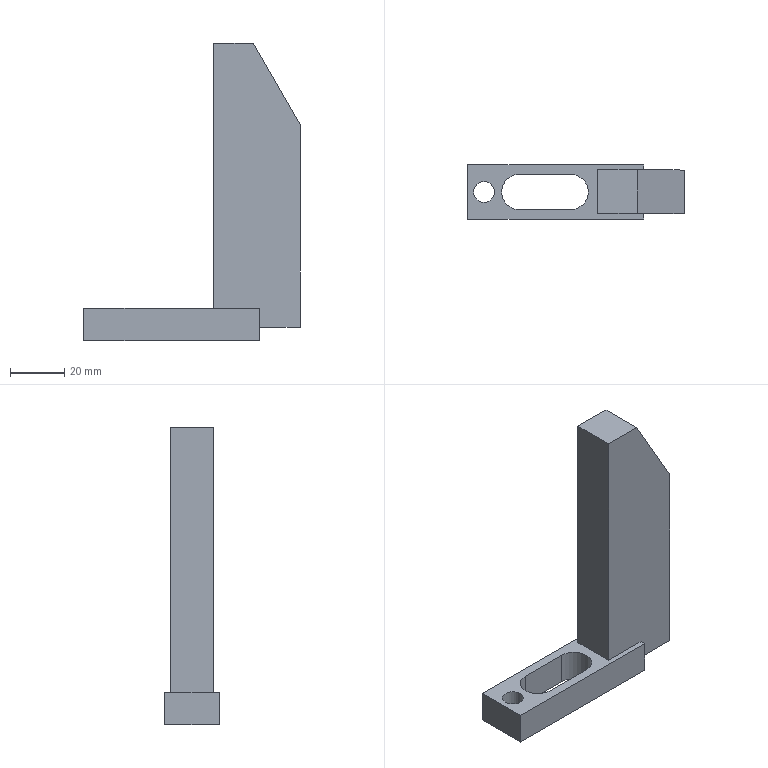Part | NX | features solid 2 | 1 solid | 18 faces | box 80 x 20 x 110 mm | volume 58169 mm3 | plane 15 | cylinder 3 | commonest cylinder face diameters 13 x2 7.8 x1
STEP:
#1=CARTESIAN_POINT('',(-633.,83.,-110.));
#2=VERTEX_POINT('',#1);
#3=CARTESIAN_POINT('',(-633.,83.,-103.));
#4=VERTEX_POINT('',#3);
#5=CARTESIAN_POINT('',(-633.,83.,-85.));
#6=DIRECTION('',(0.,0.,1.));
#7=VECTOR('',#6,1000.);
#8=LINE('',#5,#7);
#9=EDGE_CURVE('',#2,#4,#8,.T.);
#10=ORIENTED_EDGE('',*,*,#9,.T.);
#11=CARTESIAN_POINT('',(-650.,83.,-103.));
#12=VERTEX_POINT('',#11);
#13=CARTESIAN_POINT('',(-665.5,83.,-103.));
#14=DIRECTION('',(-1.,0.,0.));
#15=VECTOR('',#14,1000.);
#16=LINE('',#13,#15);
#17=EDGE_CURVE('',#4,#12,#16,.T.);
#18=ORIENTED_EDGE('',*,*,#17,.T.);
#19=CARTESIAN_POINT('',(-650.,83.,-5.));
#20=VERTEX_POINT('',#19);
#21=CARTESIAN_POINT('',(-650.,83.,-150.));
#22=DIRECTION('',(0.,0.,1.));
#23=VECTOR('',#22,1000.);
#24=LINE('',#21,#23);
#25=EDGE_CURVE('',#12,#20,#24,.T.);
#26=ORIENTED_EDGE('',*,*,#25,.T.);
#27=CARTESIAN_POINT('',(-635.321,83.,-5.));
#28=VERTEX_POINT('',#27);
#29=CARTESIAN_POINT('',(-634.,83.,-5.));
#30=DIRECTION('',(1.,0.,0.));
#31=VECTOR('',#30,1000.);
#32=LINE('',#29,#31);
#33=EDGE_CURVE('',#20,#28,#32,.T.);
#34=ORIENTED_EDGE('',*,*,#33,.T.);
#35=CARTESIAN_POINT('',(-618.,83.,-35.));
#36=VERTEX_POINT('',#35);
#37=CARTESIAN_POINT('',(-618.,83.,-35.));
#38=DIRECTION('',(-0.5,0.,0.866));
#39=VECTOR('',#38,1000.);
#40=LINE('',#37,#39);
#41=EDGE_CURVE('',#36,#28,#40,.T.);
#42=ORIENTED_EDGE('',*,*,#41,.F.);
#43=CARTESIAN_POINT('',(-618.,83.,-110.));
#44=VERTEX_POINT('',#43);
#45=CARTESIAN_POINT('',(-618.,83.,-80.));
#46=DIRECTION('',(0.,0.,1.));
#47=VECTOR('',#46,1000.);
#48=LINE('',#45,#47);
#49=EDGE_CURVE('',#44,#36,#48,.T.);
#50=ORIENTED_EDGE('',*,*,#49,.F.);
#51=CARTESIAN_POINT('',(-634.,83.,-110.));
#52=DIRECTION('',(-1.,0.,0.));
#53=VECTOR('',#52,1000.);
#54=LINE('',#51,#53);
#55=EDGE_CURVE('',#44,#2,#54,.T.);
#56=ORIENTED_EDGE('',*,*,#55,.T.);
#57=EDGE_LOOP('',(#10,#18,#26,#34,#42,#50,#56));
#58=FACE_BOUND('',#57,.T.);
#59=CARTESIAN_POINT('',(-634.,83.,-80.));
#60=DIRECTION('',(0.,1.,0.));
#61=DIRECTION('',(0.,0.,-1.));
#62=AXIS2_PLACEMENT_3D('',#59,#60,#61);
#63=PLANE('',#62);
#64=ADVANCED_FACE('',(#58),#63,.T.);
#65=ORIENTED_EDGE('',*,*,#49,.T.);
#66=CARTESIAN_POINT('',(-618.,67.,-35.));
#67=VERTEX_POINT('',#66);
#68=CARTESIAN_POINT('',(-618.,75.,-35.));
#69=DIRECTION('',(0.,-1.,0.));
#70=VECTOR('',#69,1000.);
#71=LINE('',#68,#70);
#72=EDGE_CURVE('',#36,#67,#71,.T.);
#73=ORIENTED_EDGE('',*,*,#72,.T.);
#74=CARTESIAN_POINT('',(-618.,67.,-110.));
#75=VERTEX_POINT('',#74);
#76=CARTESIAN_POINT('',(-618.,67.,-80.));
#77=DIRECTION('',(0.,0.,1.));
#78=VECTOR('',#77,1000.);
#79=LINE('',#76,#78);
#80=EDGE_CURVE('',#75,#67,#79,.T.);
#81=ORIENTED_EDGE('',*,*,#80,.F.);
#82=CARTESIAN_POINT('',(-618.,75.,-110.));
#83=DIRECTION('',(0.,1.,0.));
#84=VECTOR('',#83,1000.);
#85=LINE('',#82,#84);
#86=EDGE_CURVE('',#75,#44,#85,.T.);
#87=ORIENTED_EDGE('',*,*,#86,.T.);
#88=EDGE_LOOP('',(#65,#73,#81,#87));
#89=FACE_BOUND('',#88,.T.);
#90=CARTESIAN_POINT('',(-618.,75.,-80.));
#91=DIRECTION('',(1.,0.,0.));
#92=DIRECTION('',(0.,0.,1.));
#93=AXIS2_PLACEMENT_3D('',#90,#91,#92);
#94=PLANE('',#93);
#95=ADVANCED_FACE('',(#89),#94,.T.);
#96=ORIENTED_EDGE('',*,*,#80,.T.);
#97=CARTESIAN_POINT('',(-635.321,67.,-5.));
#98=VERTEX_POINT('',#97);
#99=CARTESIAN_POINT('',(-618.,67.,-35.));
#100=DIRECTION('',(-0.5,0.,0.866));
#101=VECTOR('',#100,1000.);
#102=LINE('',#99,#101);
#103=EDGE_CURVE('',#67,#98,#102,.T.);
#104=ORIENTED_EDGE('',*,*,#103,.T.);
#105=CARTESIAN_POINT('',(-650.,67.,-5.));
#106=VERTEX_POINT('',#105);
#107=CARTESIAN_POINT('',(-634.,67.,-5.));
#108=DIRECTION('',(-1.,0.,0.));
#109=VECTOR('',#108,1000.);
#110=LINE('',#107,#109);
#111=EDGE_CURVE('',#98,#106,#110,.T.);
#112=ORIENTED_EDGE('',*,*,#111,.T.);
#113=CARTESIAN_POINT('',(-650.,67.,-103.));
#114=VERTEX_POINT('',#113);
#115=CARTESIAN_POINT('',(-650.,67.,-150.));
#116=DIRECTION('',(0.,0.,1.));
#117=VECTOR('',#116,1000.);
#118=LINE('',#115,#117);
#119=EDGE_CURVE('',#114,#106,#118,.T.);
#120=ORIENTED_EDGE('',*,*,#119,.F.);
#121=CARTESIAN_POINT('',(-633.,67.,-103.));
#122=VERTEX_POINT('',#121);
#123=CARTESIAN_POINT('',(-665.5,67.,-103.));
#124=DIRECTION('',(1.,0.,0.));
#125=VECTOR('',#124,1000.);
#126=LINE('',#123,#125);
#127=EDGE_CURVE('',#114,#122,#126,.T.);
#128=ORIENTED_EDGE('',*,*,#127,.T.);
#129=CARTESIAN_POINT('',(-633.,67.,-110.));
#130=VERTEX_POINT('',#129);
#131=CARTESIAN_POINT('',(-633.,67.,-85.));
#132=DIRECTION('',(0.,0.,-1.));
#133=VECTOR('',#132,1000.);
#134=LINE('',#131,#133);
#135=EDGE_CURVE('',#122,#130,#134,.T.);
#136=ORIENTED_EDGE('',*,*,#135,.T.);
#137=CARTESIAN_POINT('',(-634.,67.,-110.));
#138=DIRECTION('',(1.,0.,0.));
#139=VECTOR('',#138,1000.);
#140=LINE('',#137,#139);
#141=EDGE_CURVE('',#130,#75,#140,.T.);
#142=ORIENTED_EDGE('',*,*,#141,.T.);
#143=EDGE_LOOP('',(#96,#104,#112,#120,#128,#136,#142));
#144=FACE_BOUND('',#143,.T.);
#145=CARTESIAN_POINT('',(-634.,67.,-80.));
#146=DIRECTION('',(0.,-1.,0.));
#147=DIRECTION('',(0.,0.,1.));
#148=AXIS2_PLACEMENT_3D('',#145,#146,#147);
#149=PLANE('',#148);
#150=ADVANCED_FACE('',(#144),#149,.T.);
#151=ORIENTED_EDGE('',*,*,#127,.F.);
#152=CARTESIAN_POINT('',(-650.,75.,-103.));
#153=DIRECTION('',(0.,-1.,0.));
#154=VECTOR('',#153,1000.);
#155=LINE('',#152,#154);
#156=EDGE_CURVE('',#12,#114,#155,.T.);
#157=ORIENTED_EDGE('',*,*,#156,.F.);
#158=ORIENTED_EDGE('',*,*,#17,.F.);
#159=CARTESIAN_POINT('',(-633.,85.,-103.));
#160=VERTEX_POINT('',#159);
#161=CARTESIAN_POINT('',(-633.,75.,-103.));
#162=DIRECTION('',(0.,-1.,0.));
#163=VECTOR('',#162,1000.);
#164=LINE('',#161,#163);
#165=EDGE_CURVE('',#160,#4,#164,.T.);
#166=ORIENTED_EDGE('',*,*,#165,.F.);
#167=CARTESIAN_POINT('',(-698.,85.,-103.));
#168=VERTEX_POINT('',#167);
#169=CARTESIAN_POINT('',(-665.5,85.,-103.));
#170=DIRECTION('',(1.,0.,0.));
#171=VECTOR('',#170,1000.);
#172=LINE('',#169,#171);
#173=EDGE_CURVE('',#168,#160,#172,.T.);
#174=ORIENTED_EDGE('',*,*,#173,.F.);
#175=CARTESIAN_POINT('',(-698.,65.,-103.));
#176=VERTEX_POINT('',#175);
#177=CARTESIAN_POINT('',(-698.,75.,-103.));
#178=DIRECTION('',(0.,1.,0.));
#179=VECTOR('',#178,1000.);
#180=LINE('',#177,#179);
#181=EDGE_CURVE('',#176,#168,#180,.T.);
#182=ORIENTED_EDGE('',*,*,#181,.F.);
#183=CARTESIAN_POINT('',(-633.,65.,-103.));
#184=VERTEX_POINT('',#183);
#185=CARTESIAN_POINT('',(-665.5,65.,-103.));
#186=DIRECTION('',(-1.,0.,0.));
#187=VECTOR('',#186,1000.);
#188=LINE('',#185,#187);
#189=EDGE_CURVE('',#184,#176,#188,.T.);
#190=ORIENTED_EDGE('',*,*,#189,.F.);
#191=CARTESIAN_POINT('',(-633.,75.,-103.));
#192=DIRECTION('',(0.,-1.,0.));
#193=VECTOR('',#192,1000.);
#194=LINE('',#191,#193);
#195=EDGE_CURVE('',#122,#184,#194,.T.);
#196=ORIENTED_EDGE('',*,*,#195,.F.);
#197=EDGE_LOOP('',(#151,#157,#158,#166,#174,#182,#190,#196));
#198=FACE_BOUND('',#197,.T.);
#199=CARTESIAN_POINT('',(-660.,81.5,-103.));
#200=VERTEX_POINT('',#199);
#201=CARTESIAN_POINT('',(-660.,68.5,-103.));
#202=VERTEX_POINT('',#201);
#203=CARTESIAN_POINT('',(-660.,75.,-103.));
#204=DIRECTION('',(0.,0.,-1.));
#205=DIRECTION('',(1.,0.,0.));
#206=AXIS2_PLACEMENT_3D('',#203,#204,#205);
#207=CIRCLE('',#206,6.5);
#208=EDGE_CURVE('',#200,#202,#207,.T.);
#209=ORIENTED_EDGE('',*,*,#208,.T.);
#210=CARTESIAN_POINT('',(-679.,68.5,-103.));
#211=VERTEX_POINT('',#210);
#212=CARTESIAN_POINT('',(-669.5,68.5,-103.));
#213=DIRECTION('',(-1.,0.,0.));
#214=VECTOR('',#213,1000.);
#215=LINE('',#212,#214);
#216=EDGE_CURVE('',#202,#211,#215,.T.);
#217=ORIENTED_EDGE('',*,*,#216,.T.);
#218=CARTESIAN_POINT('',(-679.,81.5,-103.));
#219=VERTEX_POINT('',#218);
#220=CARTESIAN_POINT('',(-679.,75.,-103.));
#221=DIRECTION('',(0.,0.,-1.));
#222=DIRECTION('',(1.,0.,0.));
#223=AXIS2_PLACEMENT_3D('',#220,#221,#222);
#224=CIRCLE('',#223,6.5);
#225=EDGE_CURVE('',#211,#219,#224,.T.);
#226=ORIENTED_EDGE('',*,*,#225,.T.);
#227=CARTESIAN_POINT('',(-669.5,81.5,-103.));
#228=DIRECTION('',(1.,0.,0.));
#229=VECTOR('',#228,1000.);
#230=LINE('',#227,#229);
#231=EDGE_CURVE('',#219,#200,#230,.T.);
#232=ORIENTED_EDGE('',*,*,#231,.T.);
#233=EDGE_LOOP('',(#209,#217,#226,#232));
#234=FACE_BOUND('',#233,.T.);
#235=CARTESIAN_POINT('',(-688.1,75.,-103.));
#236=VERTEX_POINT('',#235);
#237=CARTESIAN_POINT('',(-692.,75.,-103.));
#238=DIRECTION('',(0.,0.,-1.));
#239=DIRECTION('',(1.,0.,0.));
#240=AXIS2_PLACEMENT_3D('',#237,#238,#239);
#241=CIRCLE('',#240,3.9);
#242=EDGE_CURVE('',#236,#236,#241,.T.);
#243=ORIENTED_EDGE('',*,*,#242,.T.);
#244=EDGE_LOOP('',(#243));
#245=FACE_BOUND('',#244,.T.);
#246=CARTESIAN_POINT('',(-665.5,75.,-103.));
#247=DIRECTION('',(0.,0.,1.));
#248=DIRECTION('',(-1.,0.,0.));
#249=AXIS2_PLACEMENT_3D('',#246,#247,#248);
#250=PLANE('',#249);
#251=ADVANCED_FACE('',(#198,#234,#245),#250,.T.);
#252=CARTESIAN_POINT('',(-698.,85.,-115.));
#253=VERTEX_POINT('',#252);
#254=CARTESIAN_POINT('',(-698.,85.,-85.));
#255=DIRECTION('',(0.,0.,1.));
#256=VECTOR('',#255,1000.);
#257=LINE('',#254,#256);
#258=EDGE_CURVE('',#253,#168,#257,.T.);
#259=ORIENTED_EDGE('',*,*,#258,.T.);
#260=ORIENTED_EDGE('',*,*,#173,.T.);
#261=CARTESIAN_POINT('',(-633.,85.,-115.));
#262=VERTEX_POINT('',#261);
#263=CARTESIAN_POINT('',(-633.,85.,-85.));
#264=DIRECTION('',(0.,0.,1.));
#265=VECTOR('',#264,1000.);
#266=LINE('',#263,#265);
#267=EDGE_CURVE('',#262,#160,#266,.T.);
#268=ORIENTED_EDGE('',*,*,#267,.F.);
#269=CARTESIAN_POINT('',(-665.5,85.,-115.));
#270=DIRECTION('',(-1.,0.,0.));
#271=VECTOR('',#270,1000.);
#272=LINE('',#269,#271);
#273=EDGE_CURVE('',#262,#253,#272,.T.);
#274=ORIENTED_EDGE('',*,*,#273,.T.);
#275=EDGE_LOOP('',(#259,#260,#268,#274));
#276=FACE_BOUND('',#275,.T.);
#277=CARTESIAN_POINT('',(-665.5,85.,-85.));
#278=DIRECTION('',(0.,1.,0.));
#279=DIRECTION('',(0.,0.,-1.));
#280=AXIS2_PLACEMENT_3D('',#277,#278,#279);
#281=PLANE('',#280);
#282=ADVANCED_FACE('',(#276),#281,.T.);
#283=ORIENTED_EDGE('',*,*,#9,.F.);
#284=CARTESIAN_POINT('',(-633.,75.,-110.));
#285=DIRECTION('',(0.,1.,0.));
#286=VECTOR('',#285,1000.);
#287=LINE('',#284,#286);
#288=EDGE_CURVE('',#130,#2,#287,.T.);
#289=ORIENTED_EDGE('',*,*,#288,.F.);
#290=ORIENTED_EDGE('',*,*,#135,.F.);
#291=ORIENTED_EDGE('',*,*,#195,.T.);
#292=CARTESIAN_POINT('',(-633.,65.,-115.));
#293=VERTEX_POINT('',#292);
#294=CARTESIAN_POINT('',(-633.,65.,-85.));
#295=DIRECTION('',(0.,0.,1.));
#296=VECTOR('',#295,1000.);
#297=LINE('',#294,#296);
#298=EDGE_CURVE('',#293,#184,#297,.T.);
#299=ORIENTED_EDGE('',*,*,#298,.F.);
#300=CARTESIAN_POINT('',(-633.,75.,-115.));
#301=DIRECTION('',(0.,1.,0.));
#302=VECTOR('',#301,1000.);
#303=LINE('',#300,#302);
#304=EDGE_CURVE('',#293,#262,#303,.T.);
#305=ORIENTED_EDGE('',*,*,#304,.T.);
#306=ORIENTED_EDGE('',*,*,#267,.T.);
#307=ORIENTED_EDGE('',*,*,#165,.T.);
#308=EDGE_LOOP('',(#283,#289,#290,#291,#299,#305,#306,#307));
#309=FACE_BOUND('',#308,.T.);
#310=CARTESIAN_POINT('',(-633.,75.,-85.));
#311=DIRECTION('',(1.,0.,0.));
#312=DIRECTION('',(0.,0.,1.));
#313=AXIS2_PLACEMENT_3D('',#310,#311,#312);
#314=PLANE('',#313);
#315=ADVANCED_FACE('',(#309),#314,.T.);
#316=ORIENTED_EDGE('',*,*,#298,.T.);
#317=ORIENTED_EDGE('',*,*,#189,.T.);
#318=CARTESIAN_POINT('',(-698.,65.,-115.));
#319=VERTEX_POINT('',#318);
#320=CARTESIAN_POINT('',(-698.,65.,-85.));
#321=DIRECTION('',(0.,0.,1.));
#322=VECTOR('',#321,1000.);
#323=LINE('',#320,#322);
#324=EDGE_CURVE('',#319,#176,#323,.T.);
#325=ORIENTED_EDGE('',*,*,#324,.F.);
#326=CARTESIAN_POINT('',(-665.5,65.,-115.));
#327=DIRECTION('',(1.,0.,0.));
#328=VECTOR('',#327,1000.);
#329=LINE('',#326,#328);
#330=EDGE_CURVE('',#319,#293,#329,.T.);
#331=ORIENTED_EDGE('',*,*,#330,.T.);
#332=EDGE_LOOP('',(#316,#317,#325,#331));
#333=FACE_BOUND('',#332,.T.);
#334=CARTESIAN_POINT('',(-665.5,65.,-85.));
#335=DIRECTION('',(0.,-1.,0.));
#336=DIRECTION('',(0.,0.,1.));
#337=AXIS2_PLACEMENT_3D('',#334,#335,#336);
#338=PLANE('',#337);
#339=ADVANCED_FACE('',(#333),#338,.T.);
#340=CARTESIAN_POINT('',(-660.,68.5,-115.));
#341=VERTEX_POINT('',#340);
#342=CARTESIAN_POINT('',(-660.,81.5,-115.));
#343=VERTEX_POINT('',#342);
#344=CARTESIAN_POINT('',(-660.,75.,-115.));
#345=DIRECTION('',(0.,0.,1.));
#346=DIRECTION('',(-1.,0.,0.));
#347=AXIS2_PLACEMENT_3D('',#344,#345,#346);
#348=CIRCLE('',#347,6.5);
#349=EDGE_CURVE('',#341,#343,#348,.T.);
#350=ORIENTED_EDGE('',*,*,#349,.T.);
#351=CARTESIAN_POINT('',(-679.,81.5,-115.));
#352=VERTEX_POINT('',#351);
#353=CARTESIAN_POINT('',(-669.5,81.5,-115.));
#354=DIRECTION('',(-1.,0.,0.));
#355=VECTOR('',#354,1000.);
#356=LINE('',#353,#355);
#357=EDGE_CURVE('',#343,#352,#356,.T.);
#358=ORIENTED_EDGE('',*,*,#357,.T.);
#359=CARTESIAN_POINT('',(-679.,68.5,-115.));
#360=VERTEX_POINT('',#359);
#361=CARTESIAN_POINT('',(-679.,75.,-115.));
#362=DIRECTION('',(0.,0.,1.));
#363=DIRECTION('',(-1.,0.,0.));
#364=AXIS2_PLACEMENT_3D('',#361,#362,#363);
#365=CIRCLE('',#364,6.5);
#366=EDGE_CURVE('',#352,#360,#365,.T.);
#367=ORIENTED_EDGE('',*,*,#366,.T.);
#368=CARTESIAN_POINT('',(-669.5,68.5,-115.));
#369=DIRECTION('',(1.,0.,0.));
#370=VECTOR('',#369,1000.);
#371=LINE('',#368,#370);
#372=EDGE_CURVE('',#360,#341,#371,.T.);
#373=ORIENTED_EDGE('',*,*,#372,.T.);
#374=EDGE_LOOP('',(#350,#358,#367,#373));
#375=FACE_BOUND('',#374,.T.);
#376=CARTESIAN_POINT('',(-695.9,75.,-115.));
#377=VERTEX_POINT('',#376);
#378=CARTESIAN_POINT('',(-692.,75.,-115.));
#379=DIRECTION('',(0.,0.,1.));
#380=DIRECTION('',(-1.,0.,0.));
#381=AXIS2_PLACEMENT_3D('',#378,#379,#380);
#382=CIRCLE('',#381,3.9);
#383=EDGE_CURVE('',#377,#377,#382,.T.);
#384=ORIENTED_EDGE('',*,*,#383,.T.);
#385=EDGE_LOOP('',(#384));
#386=FACE_BOUND('',#385,.T.);
#387=CARTESIAN_POINT('',(-698.,75.,-115.));
#388=DIRECTION('',(0.,-1.,0.));
#389=VECTOR('',#388,1000.);
#390=LINE('',#387,#389);
#391=EDGE_CURVE('',#253,#319,#390,.T.);
#392=ORIENTED_EDGE('',*,*,#391,.F.);
#393=ORIENTED_EDGE('',*,*,#273,.F.);
#394=ORIENTED_EDGE('',*,*,#304,.F.);
#395=ORIENTED_EDGE('',*,*,#330,.F.);
#396=EDGE_LOOP('',(#392,#393,#394,#395));
#397=FACE_BOUND('',#396,.T.);
#398=CARTESIAN_POINT('',(-665.5,75.,-115.));
#399=DIRECTION('',(0.,0.,-1.));
#400=DIRECTION('',(1.,0.,0.));
#401=AXIS2_PLACEMENT_3D('',#398,#399,#400);
#402=PLANE('',#401);
#403=ADVANCED_FACE('',(#375,#386,#397),#402,.T.);
#404=ORIENTED_EDGE('',*,*,#391,.T.);
#405=ORIENTED_EDGE('',*,*,#324,.T.);
#406=ORIENTED_EDGE('',*,*,#181,.T.);
#407=ORIENTED_EDGE('',*,*,#258,.F.);
#408=EDGE_LOOP('',(#404,#405,#406,#407));
#409=FACE_BOUND('',#408,.T.);
#410=CARTESIAN_POINT('',(-698.,75.,-85.));
#411=DIRECTION('',(-1.,0.,0.));
#412=DIRECTION('',(0.,0.,-1.));
#413=AXIS2_PLACEMENT_3D('',#410,#411,#412);
#414=PLANE('',#413);
#415=ADVANCED_FACE('',(#409),#414,.T.);
#416=ORIENTED_EDGE('',*,*,#242,.F.);
#417=EDGE_LOOP('',(#416));
#418=FACE_BOUND('',#417,.T.);
#419=ORIENTED_EDGE('',*,*,#383,.F.);
#420=EDGE_LOOP('',(#419));
#421=FACE_BOUND('',#420,.T.);
#422=CARTESIAN_POINT('',(-692.,75.,-85.));
#423=DIRECTION('',(0.,0.,1.));
#424=DIRECTION('',(-1.,0.,0.));
#425=AXIS2_PLACEMENT_3D('',#422,#423,#424);
#426=CYLINDRICAL_SURFACE('',#425,3.9);
#427=ADVANCED_FACE('',(#418,#421),#426,.F.);
#428=CARTESIAN_POINT('',(-679.,81.5,-85.));
#429=DIRECTION('',(0.,0.,1.));
#430=VECTOR('',#429,1000.);
#431=LINE('',#428,#430);
#432=EDGE_CURVE('',#352,#219,#431,.T.);
#433=ORIENTED_EDGE('',*,*,#432,.F.);
#434=ORIENTED_EDGE('',*,*,#357,.F.);
#435=CARTESIAN_POINT('',(-660.,81.5,-85.));
#436=DIRECTION('',(0.,0.,1.));
#437=VECTOR('',#436,1000.);
#438=LINE('',#435,#437);
#439=EDGE_CURVE('',#343,#200,#438,.T.);
#440=ORIENTED_EDGE('',*,*,#439,.T.);
#441=ORIENTED_EDGE('',*,*,#231,.F.);
#442=EDGE_LOOP('',(#433,#434,#440,#441));
#443=FACE_BOUND('',#442,.T.);
#444=CARTESIAN_POINT('',(-669.5,81.5,-85.));
#445=DIRECTION('',(0.,1.,0.));
#446=DIRECTION('',(0.,0.,-1.));
#447=AXIS2_PLACEMENT_3D('',#444,#445,#446);
#448=PLANE('',#447);
#449=ADVANCED_FACE('',(#443),#448,.F.);
#450=CARTESIAN_POINT('',(-660.,68.5,-85.));
#451=DIRECTION('',(0.,0.,1.));
#452=VECTOR('',#451,1000.);
#453=LINE('',#450,#452);
#454=EDGE_CURVE('',#341,#202,#453,.T.);
#455=ORIENTED_EDGE('',*,*,#454,.F.);
#456=ORIENTED_EDGE('',*,*,#372,.F.);
#457=CARTESIAN_POINT('',(-679.,68.5,-85.));
#458=DIRECTION('',(0.,0.,1.));
#459=VECTOR('',#458,1000.);
#460=LINE('',#457,#459);
#461=EDGE_CURVE('',#360,#211,#460,.T.);
#462=ORIENTED_EDGE('',*,*,#461,.T.);
#463=ORIENTED_EDGE('',*,*,#216,.F.);
#464=EDGE_LOOP('',(#455,#456,#462,#463));
#465=FACE_BOUND('',#464,.T.);
#466=CARTESIAN_POINT('',(-669.5,68.5,-85.));
#467=DIRECTION('',(0.,-1.,0.));
#468=DIRECTION('',(0.,0.,1.));
#469=AXIS2_PLACEMENT_3D('',#466,#467,#468);
#470=PLANE('',#469);
#471=ADVANCED_FACE('',(#465),#470,.F.);
#472=ORIENTED_EDGE('',*,*,#349,.F.);
#473=ORIENTED_EDGE('',*,*,#454,.T.);
#474=ORIENTED_EDGE('',*,*,#208,.F.);
#475=ORIENTED_EDGE('',*,*,#439,.F.);
#476=EDGE_LOOP('',(#472,#473,#474,#475));
#477=FACE_BOUND('',#476,.T.);
#478=CARTESIAN_POINT('',(-660.,75.,-85.));
#479=DIRECTION('',(0.,0.,1.));
#480=DIRECTION('',(-1.,0.,0.));
#481=AXIS2_PLACEMENT_3D('',#478,#479,#480);
#482=CYLINDRICAL_SURFACE('',#481,6.5);
#483=ADVANCED_FACE('',(#477),#482,.F.);
#484=ORIENTED_EDGE('',*,*,#366,.F.);
#485=ORIENTED_EDGE('',*,*,#432,.T.);
#486=ORIENTED_EDGE('',*,*,#225,.F.);
#487=ORIENTED_EDGE('',*,*,#461,.F.);
#488=EDGE_LOOP('',(#484,#485,#486,#487));
#489=FACE_BOUND('',#488,.T.);
#490=CARTESIAN_POINT('',(-679.,75.,-85.));
#491=DIRECTION('',(0.,0.,1.));
#492=DIRECTION('',(-1.,0.,0.));
#493=AXIS2_PLACEMENT_3D('',#490,#491,#492);
#494=CYLINDRICAL_SURFACE('',#493,6.5);
#495=ADVANCED_FACE('',(#489),#494,.F.);
#496=ORIENTED_EDGE('',*,*,#141,.F.);
#497=ORIENTED_EDGE('',*,*,#288,.T.);
#498=ORIENTED_EDGE('',*,*,#55,.F.);
#499=ORIENTED_EDGE('',*,*,#86,.F.);
#500=EDGE_LOOP('',(#496,#497,#498,#499));
#501=FACE_BOUND('',#500,.T.);
#502=CARTESIAN_POINT('',(-634.,75.,-110.));
#503=DIRECTION('',(0.,0.,-1.));
#504=DIRECTION('',(1.,0.,0.));
#505=AXIS2_PLACEMENT_3D('',#502,#503,#504);
#506=PLANE('',#505);
#507=ADVANCED_FACE('',(#501),#506,.T.);
#508=ORIENTED_EDGE('',*,*,#25,.F.);
#509=ORIENTED_EDGE('',*,*,#156,.T.);
#510=ORIENTED_EDGE('',*,*,#119,.T.);
#511=CARTESIAN_POINT('',(-650.,75.,-5.));
#512=DIRECTION('',(0.,1.,0.));
#513=VECTOR('',#512,1000.);
#514=LINE('',#511,#513);
#515=EDGE_CURVE('',#106,#20,#514,.T.);
#516=ORIENTED_EDGE('',*,*,#515,.T.);
#517=EDGE_LOOP('',(#508,#509,#510,#516));
#518=FACE_BOUND('',#517,.T.);
#519=CARTESIAN_POINT('',(-650.,75.,-150.));
#520=DIRECTION('',(-1.,0.,0.));
#521=DIRECTION('',(0.,0.,-1.));
#522=AXIS2_PLACEMENT_3D('',#519,#520,#521);
#523=PLANE('',#522);
#524=ADVANCED_FACE('',(#518),#523,.T.);
#525=CARTESIAN_POINT('',(-635.321,75.,-5.));
#526=DIRECTION('',(0.,-1.,0.));
#527=VECTOR('',#526,1000.);
#528=LINE('',#525,#527);
#529=EDGE_CURVE('',#28,#98,#528,.T.);
#530=ORIENTED_EDGE('',*,*,#529,.T.);
#531=ORIENTED_EDGE('',*,*,#103,.F.);
#532=ORIENTED_EDGE('',*,*,#72,.F.);
#533=ORIENTED_EDGE('',*,*,#41,.T.);
#534=EDGE_LOOP('',(#530,#531,#532,#533));
#535=FACE_BOUND('',#534,.T.);
#536=CARTESIAN_POINT('',(-618.,75.,-35.));
#537=DIRECTION('',(-0.866,0.,-0.5));
#538=DIRECTION('',(0.5,0.,-0.866));
#539=AXIS2_PLACEMENT_3D('',#536,#537,#538);
#540=PLANE('',#539);
#541=ADVANCED_FACE('',(#535),#540,.F.);
#542=ORIENTED_EDGE('',*,*,#529,.F.);
#543=ORIENTED_EDGE('',*,*,#33,.F.);
#544=ORIENTED_EDGE('',*,*,#515,.F.);
#545=ORIENTED_EDGE('',*,*,#111,.F.);
#546=EDGE_LOOP('',(#542,#543,#544,#545));
#547=FACE_BOUND('',#546,.T.);
#548=CARTESIAN_POINT('',(-634.,75.,-5.));
#549=DIRECTION('',(0.,0.,1.));
#550=DIRECTION('',(-1.,0.,0.));
#551=AXIS2_PLACEMENT_3D('',#548,#549,#550);
#552=PLANE('',#551);
#553=ADVANCED_FACE('',(#547),#552,.T.);
#554=CLOSED_SHELL('',(#64,#95,#150,#251,#282,#315,#339,#403,#415,#427,#449,#471,#483,#495,#507,#524,#541,#553));
#555=MANIFOLD_SOLID_BREP('',#554);
#556=(LENGTH_UNIT()NAMED_UNIT(*)SI_UNIT(.MILLI.,.METRE.));
#557=UNCERTAINTY_MEASURE_WITH_UNIT(LENGTH_MEASURE(0.00001),#556,'','');
#558=(NAMED_UNIT(*)PLANE_ANGLE_UNIT()SI_UNIT($,.RADIAN.));
#559=(NAMED_UNIT(*)SI_UNIT($,.STERADIAN.)SOLID_ANGLE_UNIT());
#560=(GEOMETRIC_REPRESENTATION_CONTEXT(3)GLOBAL_UNCERTAINTY_ASSIGNED_CONTEXT((#557))GLOBAL_UNIT_ASSIGNED_CONTEXT((#556,#558,#559))REPRESENTATION_CONTEXT('',''));
#561=ADVANCED_BREP_SHAPE_REPRESENTATION('',(#555),#560);